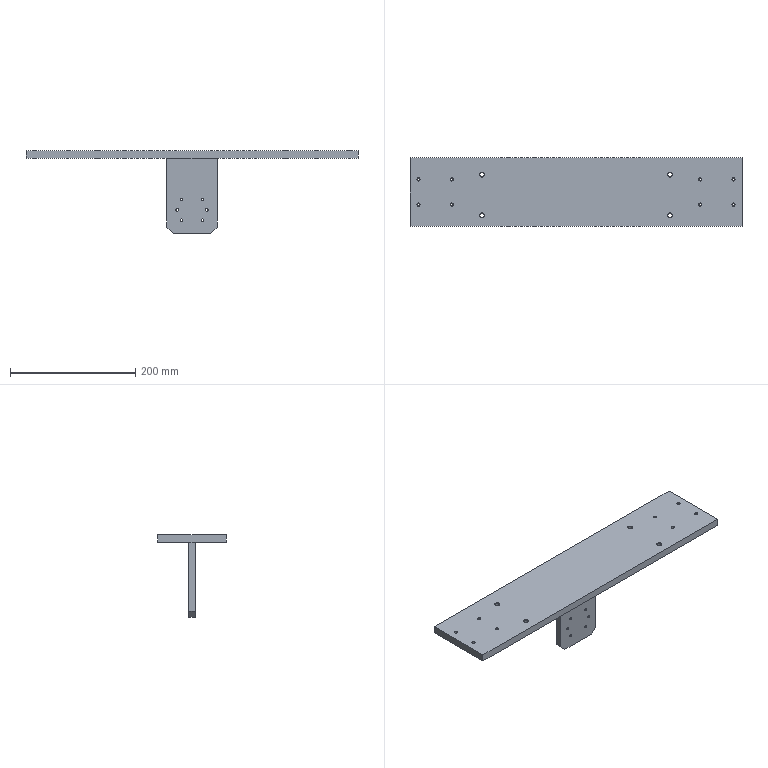Part | SolidWorks | features HoleWzd 2, Chamfer 1, Cut 1, Extrusion 1, ICE 1 | 1 solid | 73 faces | box 530 x 110 x 132 mm | volume 790668 mm3 | cylinder 36 | cone 24 | plane 13 | commonest cylinder face diameters 4.2 x28 6.8 x8